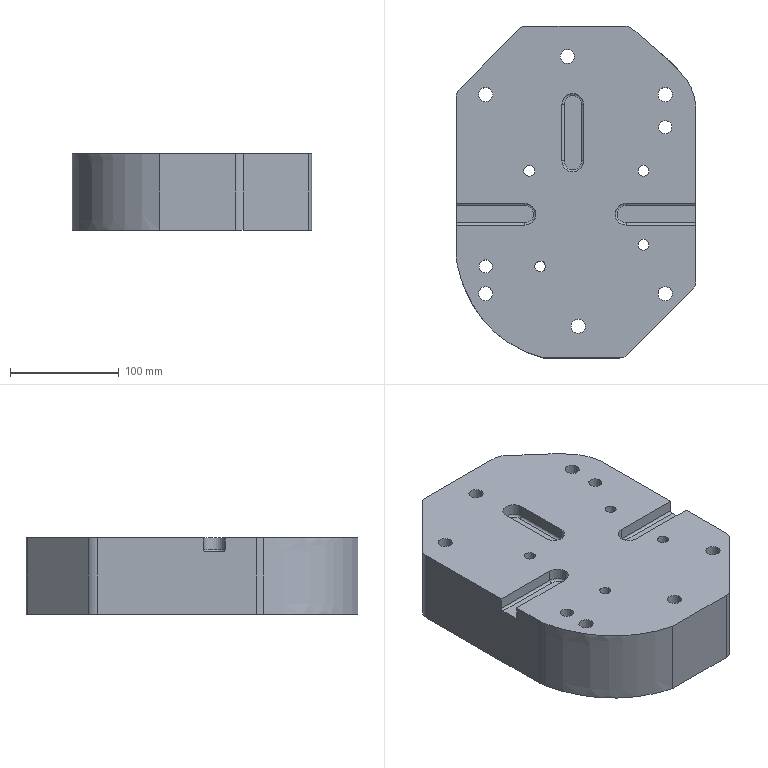Part | STEP file | 210_id2262_x_t | 1 solid | 80 faces | box 220 x 305 x 70 mm | volume 3957216 mm3 | cylinder 40 | plane 26 | cone 8 | torus 4 | other 2 | commonest cylinder face diameters 20 x12 4 x6 13 x6 8.5 x4 10 x4 12 x3